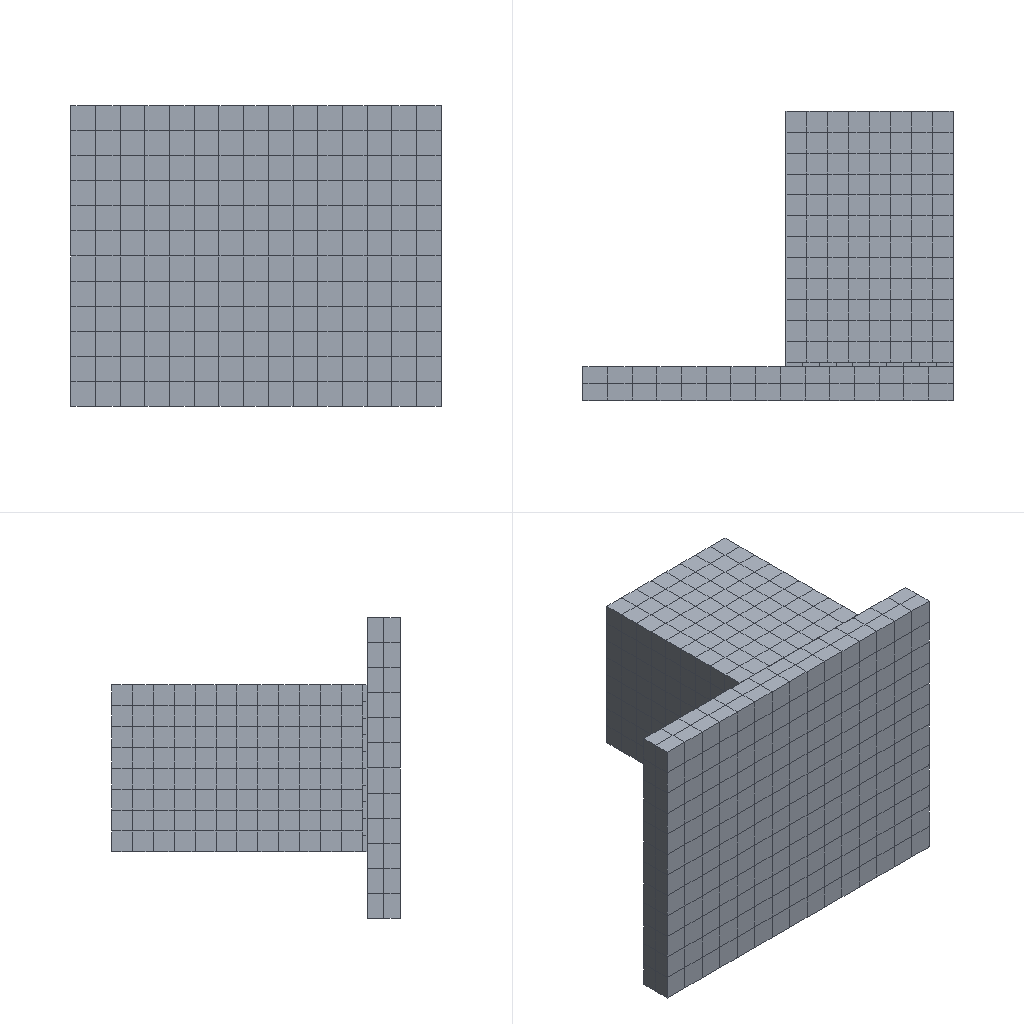Simulation study | ansys workbench
Ansys APDL input file, long lists of numbers shortened:
/batch
/config,noeldb,1     ! force off writing results to database
*get,_wallstrt,active,,time,wall
! ANSYS input file written by Workbench version 2022 R1
! File used for geometry attach:
/title,111--____ (D5)
! ****** Begin Custom Load Command Snippet ******
/COM, ACT Extensions:
/COM,     LSDYNA, 2021.1
/COM,
! ****** End   Custom Load Command Snippet ******
*DIM,_wb_ProjectScratch_dir,string,248
_wb_ProjectScratch_dir(1) = ''
*DIM,_wb_SolverFiles_dir,string,248
_wb_SolverFiles_dir(1) = ''
*DIM,_wb_userfiles_dir,string,248
_wb_userfiles_dir(1) = ''
/com,--- Data in consistent NMM units. See Solving Units in the help system for more information.
/units,MPA
/nopr
/wb,file,start              !  signify a WB generated input file
/prep7
! Turn off shape checking because checks already performed inside WB mesher.
! See help system for more information.
SHPP,OFF,,NOWARN
/nolist
etcon,set             ! allow ANSYS to choose best KEYOP's for 180x elements, resets any applicable keyopt to MAPDL defaults
/com,*********** Nodes for the whole assembly ***********
nblock,3,,7591
(1i9,3e20.9e3)
        1    -2.000000000E+00     0.000000000E+00    -2.000000000E+00
! (6900 more lines like these left out)
-1
/wb,elem,start            !  set before creation of elements
/com,*********** Elements for Body 1 "__2____1|NONE" ***********
et,1,186
keyo,1,2,1          ! set full integration on SOLID186
eblock,19,solid,,768
(19i9)
        1        1        1        1        0        0        0        0       20        0      461     3005     3858     3875     3882     3620     3859     3874     3959
! (1535 more lines like these left out)
-1
/com,*********** Elements for Body 2 "__5____1|NONE" ***********
et,2,186
keyo,2,2,1          ! set full integration on SOLID186
eblock,19,solid,,360
(19i9)
        2        2        2        2        0        0        0        0       20        0      101      804     1320     1348     1416     1111     1347     1349     1417
! (719 more lines like these left out)
-1
/com,*********** Elements for Body 3 "__3^___1|__-__1" ***********
et,3,186
keyo,3,2,1          ! set full integration on SOLID186
eblock,19,solid,,100
(19i9)
        3        3        3        3        0        0        0        0       20        0        1       81      222      223      224       82      183      182      181
! (199 more lines like these left out)
-1
/wb,elem,end               !  done creating elements
/com,*********** Send User Defined Coordinate System(s) ***********
csys,0
toffst,273.15,  ! Temperature offset from absolute zero
/com,*********** Set Reference Temperature ***********
tref,22.
/wb,mat,start              !  starting to send materials
/com,*********** Send Materials ***********
Temperature = 'TEMP' ! Temperature
MP,DENS,1,7.85e-09,	! tonne mm^-3
MP,ALPX,1,1.2e-05,	! C^-1
MP,C,1,434000000,	! mm^2 s^-2 C^-1
MP,KXX,1,60.5,	! tonne mm s^-3 C^-1
MP,RSVX,1,0.00017,	! ohm mm
MP,EX,1,200000,	! tonne s^-2 mm^-1
MP,NUXY,1,0.3,
MP,MURX,1,10000,
Temperature = 'TEMP' ! Temperature
MP,DENS,2,7.85e-09,	! tonne mm^-3
MP,ALPX,2,1.2e-05,	! C^-1
MP,C,2,434000000,	! mm^2 s^-2 C^-1
MP,KXX,2,60.5,	! tonne mm s^-3 C^-1
MP,RSVX,2,0.00017,	! ohm mm
MP,EX,2,200000,	! tonne s^-2 mm^-1
MP,NUXY,2,0.3,
MP,MURX,2,10000,
Temperature = 'TEMP' ! Temperature
MP,DENS,3,7.85e-09,	! tonne mm^-3
MP,ALPX,3,1.2e-05,	! C^-1
MP,C,3,434000000,	! mm^2 s^-2 C^-1
MP,KXX,3,60.5,	! tonne mm s^-3 C^-1
MP,RSVX,3,0.00017,	! ohm mm
MP,EX,3,200000,	! tonne s^-2 mm^-1
MP,NUXY,3,0.3,
MP,MURX,3,10000,
/wb,mat,end                !  done sending materials
!************************* Model Summary ********************
!__2____1|NONE,	结构钢,	matid,	1
!__5____1|NONE,	结构钢,	matid,	2
!__3^___1|__-__1,	结构钢,	matid,	3
!************************* End Model Summary ********************
! get the diagonal of the bounding box. Needed later for other things
*get,_xmin,node,,mnloc,x
*get,_ymin,node,,mnloc,y
*get,_zmin,node,,mnloc,z
*get,_xmax,node,,mxloc,x
*get,_ymax,node,,mxloc,y
*get,_zmax,node,,mxloc,z
_ASMDIAG=(_xmax-_xmin)*(_xmax-_xmin)+(_ymax-_ymin)*(_ymax-_ymin)+(_zmax-_zmin)*(_zmax-_zmin)
_ASMDIAG=SQRT(_ASMDIAG)
/wb,contact,start          !  starting to send contact
/com,*********** Create Contact "接触区域" ***********
/com,            Real Constant Set For Above Contact Is 5 & 4
*set,tid,5
*set,cid,4
r,tid
r,cid
et,tid,170
et,cid,174
eblock,10,,,64
(15i9)
     2449        5        5        5        0     3730     3738     3809     3729     6288     6304     6286     6285
! (63 more lines like these left out)
-1
eblock,10,,,64
(15i9)
     2513        4        4        4        0     3730     3738     3809     3729     6288     6304     6286     6285
! (63 more lines like these left out)
-1
eblock,10,,,100
(15i9)
     2577        4        5        4        0      222       81      224      223      502      503      785      784
! (99 more lines like these left out)
-1
eblock,10,,,100
(15i9)
     2677        5        4        5        0      222       81      224      223      502      503      785      784
! (99 more lines like these left out)
-1
keyo,cid,8,2               ! auto create asymmetric contact (from Program Controlled setting)
keyo,cid,10,0              ! adjust contact stiffness each NR iteration (from Program Controlled setting)
keyo,cid,12,5              ! bonded always
keyo,cid,2,0               ! augmented Lagrange
keyo,cid,4,0               ! on Gauss point (from Program Controlled setting)
keyo,cid,9,1               ! ignore initial gaps/penetration
keyo,cid,7,0               ! No Prediction
rmod,tid,3,10.      ! FKN
rmod,tid,5,0.       ! ICONT
rmod,tid,6,0.       ! PINB
rmod,tid,10,0.      ! CNOF
rmod,tid,12,0.      ! FKT
rmod,tid,36,33      ! WB DSID
rmod,cid,3,10.      ! FKN
rmod,cid,5,0.       ! ICONT
rmod,cid,6,0.       ! PINB
rmod,cid,10,0.      ! CNOF
rmod,cid,12,0.      ! FKT
rmod,cid,36,33      ! WB DSID
/com,*********** Create Contact "接触区域 2" ***********
/com,            Real Constant Set For Above Contact Is 7 & 6
*set,tid,7
*set,cid,6
r,tid
r,cid
et,tid,170
et,cid,174
eblock,10,,,56
(15i9)
     2777        7        7        7        0     1201     1202     1191     1190     2600     2580     2577     2578
! (55 more lines like these left out)
-1
eblock,10,,,56
(15i9)
     2833        6        6        6        0     1201     1202     1191     1190     2600     2580     2577     2578
! (55 more lines like these left out)
-1
eblock,10,,,100
(15i9)
     2889        6        7        6        0      181       82      183      182      506      507      723      721
! (99 more lines like these left out)
-1
eblock,10,,,100
(15i9)
     2989        7        6        7        0      181       82      183      182      506      507      723      721
! (99 more lines like these left out)
-1
keyo,cid,8,2               ! auto create asymmetric contact (from Program Controlled setting)
keyo,cid,10,0              ! adjust contact stiffness each NR iteration (from Program Controlled setting)
keyo,cid,12,5              ! bonded always
keyo,cid,2,0               ! augmented Lagrange
keyo,cid,4,0               ! on Gauss point (from Program Controlled setting)
keyo,cid,9,1               ! ignore initial gaps/penetration
keyo,cid,7,0               ! No Prediction
rmod,tid,3,10.      ! FKN
rmod,tid,5,0.       ! ICONT
rmod,tid,6,0.       ! PINB
rmod,tid,10,0.      ! CNOF
rmod,tid,12,0.      ! FKT
rmod,tid,36,36      ! WB DSID
rmod,cid,3,10.      ! FKN
rmod,cid,5,0.       ! ICONT
rmod,cid,6,0.       ! PINB
rmod,cid,10,0.      ! CNOF
rmod,cid,12,0.      ! FKT
rmod,cid,36,36      ! WB DSID
nsel,all
esel,all
/wb,contact,end            !  done creating contacts
/com,*********** Create Debonding "____" ***********
TB,CZM,4,1,,CBDE
TBDATA,1,1e-07,5e-06,8e-09,5e-06,0.1,0
TBDATA,7,2
*set,matid,4
/com,*********** Create Debonding "____ 2" ***********
TB,CZM,6,1,,CBDE
TBDATA,1,1e-07,5e-06,8e-09,5e-06,0.1,0
TBDATA,7,2
*set,matid,6
/golist
/wb,load,start             !  starting to send loads
/com,*********** Fixed Supports ***********
CMBLOCK,_FIXEDSU,NODE,      595
(8i10)
       958       959       960       961       962       963       964       965
! (74 more lines like these left out)
cmsel,s,_FIXEDSU
d,all,all
nsel,all
/com,*********** Define Force Using Surface Effect Elements ***********
local,12,0,0.,0.,0.,0.,0.,0.
csys,0
et,8,154
eblock,10,,,106
(15i9)
     3089        8        8        8       12     3721     3621     3719     3720     6053     6052     6266     6268
! (105 more lines like these left out)
-1
esel,s,type,,8
keyop,8,2,1                ! Apply load in local coordinate system
keyop,8,7,1                ! Use original area so load is constant in large deformation
esel,all
/gst,on,on
fini
*get,_numnode,node,0,count
*get,_numelem,elem,0,count
*get, _MAXELEMNUM, elem, 0, NUM, MAX
*get, _MAXNODENUM, node, 0, NUM, MAX
*get, _MAXELEMTYPE, etyp, 0, NUM, MAX
*get, _MAXREALCONST, real, 0, NUM, MAX
/go
/wb,load,end               !  done creating loads
/com,--- Number of total nodes = %_numnode%
/com,--- Number of contact elements = 746
/com,--- Number of spring elements = 0
/com,--- Number of bearing elements = 0
/com,--- Number of solid elements = 1228
/com,--- Number of condensed parts = 0
/com,--- Number of total elements = %_numelem%
*get,_wallbsol,active,,time,wall
/com,****************************************************************************
/com,*************************    SOLUTION       ********************************
/com,****************************************************************************
/solu
antype,0                   ! static analysis
_thickRatio=0.333   ! Ratio of thick parts in the model
eqsl,sparse,,,,,1
cntr,print,1               ! print out contact info and also make no initial contact an error
dmpoption,emat,no             ! Don't combine emat file for DANSYS
dmpoption,esav,no             ! Don't combine esav file for DANSYS
nldiag,cont,iter           ! print out contact info each equilibrium iteration
rescontrol,define,last,last,,dele	   ! Program Controlled
/com,****************************************************
/com,******************* SOLVE FOR LS 1 OF 1 ****************
esel,s,type,,8
nsle
sfe,all,1,pres,1,13.089
sfe,all,2,pres,1,0.
sfe,all,3,pres,1,-2.2705804659384e-015
nsel,all
esel,all
/nopr
/gopr
autots,on                  ! Workbench Program Controlled automatic time stepping
nsub,5,1000,1              ! due to presence of nonlinear materials
time,1.
outres,erase
outres,all,none
outres,nsol,all,
outres,rsol,all
outres,eangl,all
outres,etmp,all
outres,veng,all
outres,strs,all,
outres,epel,all,
outres,eppl,all,
outres,cont,all,
! *********** WB SOLVE COMMAND ***********
! check interactive state
*get,ANSINTER_,active,,int
*if,ANSINTER_,ne,0,then
/eof
*endif
solve
/com *************** Write FE CONNECTORS *********
CEWRITE,file,ce,,INTE
/com,****************************************************
/com,*************** FINISHED SOLVE FOR LS 1 *************
*get,_wallasol,active,,time,wall
/nopr
*get,_numnode,node,0,count
*get,_numelem,elem,0,count
*get, _MAXELEMNUM, elem, 0, NUM, MAX
*get, _MAXNODENUM, node, 0, NUM, MAX,,,INTERNAL
*get, _MAXELEMTYPE, etyp, 0, NUM, MAX
*get, _MAXREALCONST, real, 0, NUM, MAX
/gopr
/post1
xmlo,ENCODING,ISO-8859-1
xmlo,parm
/xml,parm,xml
fini
/gopr
*get,_walldone,active,,time,wall
_preptime=(_wallbsol-_wallstrt)*3600
_solvtime=(_wallasol-_wallbsol)*3600
_posttime=(_walldone-_wallasol)*3600
_totaltim=(_walldone-_wallstrt)*3600
*get,_dlbratio,active,0,solu,dlbr
*get,_combtime,active,0,solu,comb
*get,_ssmode,active,0,solu,ssmm
*get,_ndofs,active,0,solu,ndof
*get,_sol_end_time,active,0,set,time
*if,_sol_end_time,eq,1.,then
/fclean				!clean distributed files
*endif
/com,--- Total number of nodes = %_numnode%
/com,--- Total number of elements = %_numelem%
/com,--- Element load balance ratio = %_dlbratio%
/com,--- Time to combine distributed files = %_combtime%
/com,--- Sparse memory mode = %_ssmode%
/com,--- Number of DOF = %_ndofs%
/wb,file,end               ! done with WB generated input